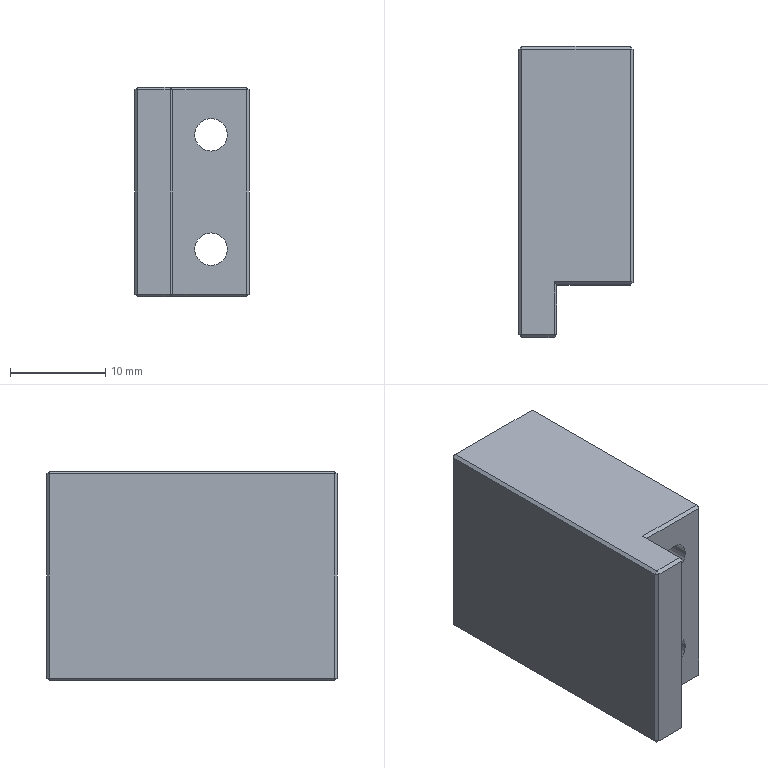Part | NX | features BREP 1 | 1 solid | 43 faces | box 12 x 30.5 x 22 mm | volume 6571 mm3 | plane 35 | cone 4 | cylinder 4 | commonest cylinder face diameters 3.4 x4
STEP:
#1=CARTESIAN_POINT('',(-3.7,-5.2,11.));
#2=VERTEX_POINT('',#1);
#3=CARTESIAN_POINT('',(-3.7,-5.5,10.7));
#4=VERTEX_POINT('',#3);
#5=CARTESIAN_POINT('',(-3.7,-5.5,10.7));
#6=DIRECTION('',(0.,-0.7071,-0.7071));
#7=VECTOR('',#6,1000.);
#8=LINE('',#5,#7);
#9=EDGE_CURVE('',#2,#4,#8,.T.);
#10=ORIENTED_EDGE('',*,*,#9,.T.);
#11=CARTESIAN_POINT('',(-0.3,-5.5,10.7));
#12=VERTEX_POINT('',#11);
#13=CARTESIAN_POINT('',(-4.,-5.5,10.7));
#14=DIRECTION('',(-1.,0.,0.));
#15=VECTOR('',#14,1000.);
#16=LINE('',#13,#15);
#17=EDGE_CURVE('',#12,#4,#16,.T.);
#18=ORIENTED_EDGE('',*,*,#17,.F.);
#19=CARTESIAN_POINT('',(-0.3,-5.2,11.));
#20=VERTEX_POINT('',#19);
#21=CARTESIAN_POINT('',(-0.3,-5.2,11.));
#22=DIRECTION('',(0.,0.7071,0.7071));
#23=VECTOR('',#22,1000.);
#24=LINE('',#21,#23);
#25=EDGE_CURVE('',#12,#20,#24,.T.);
#26=ORIENTED_EDGE('',*,*,#25,.T.);
#27=CARTESIAN_POINT('',(0.,-5.2,11.));
#28=DIRECTION('',(1.,0.,0.));
#29=VECTOR('',#28,1000.);
#30=LINE('',#27,#29);
#31=EDGE_CURVE('',#2,#20,#30,.T.);
#32=ORIENTED_EDGE('',*,*,#31,.F.);
#33=EDGE_LOOP('',(#10,#18,#26,#32));
#34=FACE_BOUND('',#33,.T.);
#35=CARTESIAN_POINT('',(0.,-5.2,11.));
#36=DIRECTION('',(0.,0.7071,-0.7071));
#37=DIRECTION('',(1.,0.,0.));
#38=AXIS2_PLACEMENT_3D('',#35,#36,#37);
#39=PLANE('',#38);
#40=ADVANCED_FACE('',(#34),#39,.F.);
#41=CARTESIAN_POINT('',(0.,-5.2,10.7));
#42=VERTEX_POINT('',#41);
#43=CARTESIAN_POINT('',(-0.15,-5.35,10.7));
#44=DIRECTION('',(0.7071,0.7071,0.));
#45=VECTOR('',#44,1000.);
#46=LINE('',#43,#45);
#47=EDGE_CURVE('',#12,#42,#46,.T.);
#48=ORIENTED_EDGE('',*,*,#47,.T.);
#49=CARTESIAN_POINT('',(-0.3,-5.2,11.));
#50=DIRECTION('',(-0.7071,0.,0.7071));
#51=VECTOR('',#50,1000.);
#52=LINE('',#49,#51);
#53=EDGE_CURVE('',#42,#20,#52,.T.);
#54=ORIENTED_EDGE('',*,*,#53,.T.);
#55=ORIENTED_EDGE('',*,*,#25,.F.);
#56=EDGE_LOOP('',(#48,#54,#55));
#57=FACE_BOUND('',#56,.T.);
#58=CARTESIAN_POINT('',(-0.3,-5.2,11.));
#59=DIRECTION('',(0.5774,-0.5774,0.5774));
#60=DIRECTION('',(0.7071,0.,-0.7071));
#61=AXIS2_PLACEMENT_3D('',#58,#59,#60);
#62=PLANE('',#61);
#63=ADVANCED_FACE('',(#57),#62,.T.);
#64=CARTESIAN_POINT('',(-4.,-5.2,10.7));
#65=VERTEX_POINT('',#64);
#66=CARTESIAN_POINT('',(-3.85,-5.2,10.85));
#67=DIRECTION('',(-0.7071,0.,-0.7071));
#68=VECTOR('',#67,1000.);
#69=LINE('',#66,#68);
#70=EDGE_CURVE('',#2,#65,#69,.T.);
#71=ORIENTED_EDGE('',*,*,#70,.T.);
#72=CARTESIAN_POINT('',(-3.7,-5.5,10.7));
#73=DIRECTION('',(0.7071,-0.7071,0.));
#74=VECTOR('',#73,1000.);
#75=LINE('',#72,#74);
#76=EDGE_CURVE('',#65,#4,#75,.T.);
#77=ORIENTED_EDGE('',*,*,#76,.T.);
#78=ORIENTED_EDGE('',*,*,#9,.F.);
#79=EDGE_LOOP('',(#71,#77,#78));
#80=FACE_BOUND('',#79,.T.);
#81=CARTESIAN_POINT('',(-3.7,-5.5,10.7));
#82=DIRECTION('',(-0.5774,-0.5774,0.5774));
#83=DIRECTION('',(0.7071,0.,0.7071));
#84=AXIS2_PLACEMENT_3D('',#81,#82,#83);
#85=PLANE('',#84);
#86=ADVANCED_FACE('',(#80),#85,.T.);
#87=CARTESIAN_POINT('',(-0.3,-5.5,-10.7));
#88=VERTEX_POINT('',#87);
#89=CARTESIAN_POINT('',(0.,-5.2,-10.7));
#90=VERTEX_POINT('',#89);
#91=CARTESIAN_POINT('',(-0.15,-5.35,-10.7));
#92=DIRECTION('',(0.7071,0.7071,0.));
#93=VECTOR('',#92,1000.);
#94=LINE('',#91,#93);
#95=EDGE_CURVE('',#88,#90,#94,.T.);
#96=ORIENTED_EDGE('',*,*,#95,.T.);
#97=CARTESIAN_POINT('',(0.,-5.2,11.));
#98=DIRECTION('',(0.,0.,-1.));
#99=VECTOR('',#98,1000.);
#100=LINE('',#97,#99);
#101=EDGE_CURVE('',#42,#90,#100,.T.);
#102=ORIENTED_EDGE('',*,*,#101,.F.);
#103=ORIENTED_EDGE('',*,*,#47,.F.);
#104=CARTESIAN_POINT('',(-0.3,-5.5,11.));
#105=DIRECTION('',(0.,0.,1.));
#106=VECTOR('',#105,1000.);
#107=LINE('',#104,#106);
#108=EDGE_CURVE('',#88,#12,#107,.T.);
#109=ORIENTED_EDGE('',*,*,#108,.F.);
#110=EDGE_LOOP('',(#96,#102,#103,#109));
#111=FACE_BOUND('',#110,.T.);
#112=CARTESIAN_POINT('',(0.,-5.2,11.));
#113=DIRECTION('',(-0.7071,0.7071,0.));
#114=DIRECTION('',(0.,0.,-1.));
#115=AXIS2_PLACEMENT_3D('',#112,#113,#114);
#116=PLANE('',#115);
#117=ADVANCED_FACE('',(#111),#116,.F.);
#118=CARTESIAN_POINT('',(0.,0.,10.7));
#119=VERTEX_POINT('',#118);
#120=CARTESIAN_POINT('',(-0.3,0.3,11.));
#121=VERTEX_POINT('',#120);
#122=CARTESIAN_POINT('',(-0.2,0.2,10.9));
#123=DIRECTION('',(-0.5774,0.5774,0.5774));
#124=VECTOR('',#123,1000.);
#125=LINE('',#122,#124);
#126=EDGE_CURVE('',#119,#121,#125,.T.);
#127=ORIENTED_EDGE('',*,*,#126,.T.);
#128=CARTESIAN_POINT('',(-0.3,0.,11.));
#129=DIRECTION('',(0.,1.,0.));
#130=VECTOR('',#129,1000.);
#131=LINE('',#128,#130);
#132=EDGE_CURVE('',#20,#121,#131,.T.);
#133=ORIENTED_EDGE('',*,*,#132,.F.);
#134=ORIENTED_EDGE('',*,*,#53,.F.);
#135=CARTESIAN_POINT('',(0.,-5.5,10.7));
#136=DIRECTION('',(0.,-1.,0.));
#137=VECTOR('',#136,1000.);
#138=LINE('',#135,#137);
#139=EDGE_CURVE('',#119,#42,#138,.T.);
#140=ORIENTED_EDGE('',*,*,#139,.F.);
#141=EDGE_LOOP('',(#127,#133,#134,#140));
#142=FACE_BOUND('',#141,.T.);
#143=CARTESIAN_POINT('',(-0.3,0.,11.));
#144=DIRECTION('',(-0.7071,0.,-0.7071));
#145=DIRECTION('',(0.,1.,0.));
#146=AXIS2_PLACEMENT_3D('',#143,#144,#145);
#147=PLANE('',#146);
#148=ADVANCED_FACE('',(#142),#147,.F.);
#149=CARTESIAN_POINT('',(-3.7,24.7,11.));
#150=VERTEX_POINT('',#149);
#151=CARTESIAN_POINT('',(-4.,24.7,10.7));
#152=VERTEX_POINT('',#151);
#153=CARTESIAN_POINT('',(-3.7,24.7,11.));
#154=DIRECTION('',(-0.7071,0.,-0.7071));
#155=VECTOR('',#154,1000.);
#156=LINE('',#153,#155);
#157=EDGE_CURVE('',#150,#152,#156,.T.);
#158=ORIENTED_EDGE('',*,*,#157,.T.);
#159=CARTESIAN_POINT('',(-4.,25.,10.7));
#160=DIRECTION('',(0.,1.,0.));
#161=VECTOR('',#160,1000.);
#162=LINE('',#159,#161);
#163=EDGE_CURVE('',#65,#152,#162,.T.);
#164=ORIENTED_EDGE('',*,*,#163,.F.);
#165=ORIENTED_EDGE('',*,*,#70,.F.);
#166=CARTESIAN_POINT('',(-3.7,0.,11.));
#167=DIRECTION('',(0.,-1.,0.));
#168=VECTOR('',#167,1000.);
#169=LINE('',#166,#168);
#170=EDGE_CURVE('',#150,#2,#169,.T.);
#171=ORIENTED_EDGE('',*,*,#170,.F.);
#172=EDGE_LOOP('',(#158,#164,#165,#171));
#173=FACE_BOUND('',#172,.T.);
#174=CARTESIAN_POINT('',(-3.7,0.,11.));
#175=DIRECTION('',(0.7071,0.,-0.7071));
#176=DIRECTION('',(0.,-1.,0.));
#177=AXIS2_PLACEMENT_3D('',#174,#175,#176);
#178=PLANE('',#177);
#179=ADVANCED_FACE('',(#173),#178,.F.);
#180=CARTESIAN_POINT('',(-4.,-5.2,-10.7));
#181=VERTEX_POINT('',#180);
#182=CARTESIAN_POINT('',(-3.7,-5.5,-10.7));
#183=VERTEX_POINT('',#182);
#184=CARTESIAN_POINT('',(-3.85,-5.35,-10.7));
#185=DIRECTION('',(0.7071,-0.7071,0.));
#186=VECTOR('',#185,1000.);
#187=LINE('',#184,#186);
#188=EDGE_CURVE('',#181,#183,#187,.T.);
#189=ORIENTED_EDGE('',*,*,#188,.T.);
#190=CARTESIAN_POINT('',(-3.7,-5.5,11.));
#191=DIRECTION('',(0.,0.,-1.));
#192=VECTOR('',#191,1000.);
#193=LINE('',#190,#192);
#194=EDGE_CURVE('',#4,#183,#193,.T.);
#195=ORIENTED_EDGE('',*,*,#194,.F.);
#196=ORIENTED_EDGE('',*,*,#76,.F.);
#197=CARTESIAN_POINT('',(-4.,-5.2,11.));
#198=DIRECTION('',(0.,0.,1.));
#199=VECTOR('',#198,1000.);
#200=LINE('',#197,#199);
#201=EDGE_CURVE('',#181,#65,#200,.T.);
#202=ORIENTED_EDGE('',*,*,#201,.F.);
#203=EDGE_LOOP('',(#189,#195,#196,#202));
#204=FACE_BOUND('',#203,.T.);
#205=CARTESIAN_POINT('',(-3.7,-5.5,11.));
#206=DIRECTION('',(0.7071,0.7071,0.));
#207=DIRECTION('',(0.,0.,-1.));
#208=AXIS2_PLACEMENT_3D('',#205,#206,#207);
#209=PLANE('',#208);
#210=ADVANCED_FACE('',(#204),#209,.F.);
#211=CARTESIAN_POINT('',(-0.3,-5.2,-11.));
#212=VERTEX_POINT('',#211);
#213=CARTESIAN_POINT('',(-0.3,-5.2,-11.));
#214=DIRECTION('',(0.,0.7071,-0.7071));
#215=VECTOR('',#214,1000.);
#216=LINE('',#213,#215);
#217=EDGE_CURVE('',#88,#212,#216,.T.);
#218=ORIENTED_EDGE('',*,*,#217,.T.);
#219=CARTESIAN_POINT('',(-0.3,-5.2,-11.));
#220=DIRECTION('',(0.7071,0.,0.7071));
#221=VECTOR('',#220,1000.);
#222=LINE('',#219,#221);
#223=EDGE_CURVE('',#212,#90,#222,.T.);
#224=ORIENTED_EDGE('',*,*,#223,.T.);
#225=ORIENTED_EDGE('',*,*,#95,.F.);
#226=EDGE_LOOP('',(#218,#224,#225));
#227=FACE_BOUND('',#226,.T.);
#228=CARTESIAN_POINT('',(-0.3,-5.2,-11.));
#229=DIRECTION('',(0.5774,-0.5774,-0.5774));
#230=DIRECTION('',(-0.7071,0.,-0.7071));
#231=AXIS2_PLACEMENT_3D('',#228,#229,#230);
#232=PLANE('',#231);
#233=ADVANCED_FACE('',(#227),#232,.T.);
#234=CARTESIAN_POINT('',(7.7,0.,10.7));
#235=VERTEX_POINT('',#234);
#236=CARTESIAN_POINT('',(7.7,0.3,11.));
#237=VERTEX_POINT('',#236);
#238=CARTESIAN_POINT('',(7.7,0.15,10.85));
#239=DIRECTION('',(0.,0.7071,0.7071));
#240=VECTOR('',#239,1000.);
#241=LINE('',#238,#240);
#242=EDGE_CURVE('',#235,#237,#241,.T.);
#243=ORIENTED_EDGE('',*,*,#242,.T.);
#244=CARTESIAN_POINT('',(0.,0.3,11.));
#245=DIRECTION('',(1.,0.,0.));
#246=VECTOR('',#245,1000.);
#247=LINE('',#244,#246);
#248=EDGE_CURVE('',#121,#237,#247,.T.);
#249=ORIENTED_EDGE('',*,*,#248,.F.);
#250=ORIENTED_EDGE('',*,*,#126,.F.);
#251=CARTESIAN_POINT('',(0.,0.,10.7));
#252=DIRECTION('',(-1.,0.,0.));
#253=VECTOR('',#252,1000.);
#254=LINE('',#251,#253);
#255=EDGE_CURVE('',#235,#119,#254,.T.);
#256=ORIENTED_EDGE('',*,*,#255,.F.);
#257=EDGE_LOOP('',(#243,#249,#250,#256));
#258=FACE_BOUND('',#257,.T.);
#259=CARTESIAN_POINT('',(0.,0.3,11.));
#260=DIRECTION('',(0.,0.7071,-0.7071));
#261=DIRECTION('',(1.,0.,0.));
#262=AXIS2_PLACEMENT_3D('',#259,#260,#261);
#263=PLANE('',#262);
#264=ADVANCED_FACE('',(#258),#263,.F.);
#265=CARTESIAN_POINT('',(-3.7,25.,10.7));
#266=VERTEX_POINT('',#265);
#267=CARTESIAN_POINT('',(-3.7,24.7,11.));
#268=DIRECTION('',(0.,0.7071,-0.7071));
#269=VECTOR('',#268,1000.);
#270=LINE('',#267,#269);
#271=EDGE_CURVE('',#150,#266,#270,.T.);
#272=ORIENTED_EDGE('',*,*,#271,.T.);
#273=CARTESIAN_POINT('',(-3.85,24.85,10.7));
#274=DIRECTION('',(-0.7071,-0.7071,0.));
#275=VECTOR('',#274,1000.);
#276=LINE('',#273,#275);
#277=EDGE_CURVE('',#266,#152,#276,.T.);
#278=ORIENTED_EDGE('',*,*,#277,.T.);
#279=ORIENTED_EDGE('',*,*,#157,.F.);
#280=EDGE_LOOP('',(#272,#278,#279));
#281=FACE_BOUND('',#280,.T.);
#282=CARTESIAN_POINT('',(-3.7,24.7,11.));
#283=DIRECTION('',(-0.5774,0.5774,0.5774));
#284=DIRECTION('',(0.7071,0.,0.7071));
#285=AXIS2_PLACEMENT_3D('',#282,#283,#284);
#286=PLANE('',#285);
#287=ADVANCED_FACE('',(#281),#286,.T.);
#288=CARTESIAN_POINT('',(-3.7,-5.2,-11.));
#289=VERTEX_POINT('',#288);
#290=CARTESIAN_POINT('',(-3.7,-5.2,-11.));
#291=DIRECTION('',(0.7071,0.,-0.7071));
#292=VECTOR('',#291,1000.);
#293=LINE('',#290,#292);
#294=EDGE_CURVE('',#181,#289,#293,.T.);
#295=ORIENTED_EDGE('',*,*,#294,.T.);
#296=CARTESIAN_POINT('',(-3.7,-5.2,-11.));
#297=DIRECTION('',(0.,-0.7071,0.7071));
#298=VECTOR('',#297,1000.);
#299=LINE('',#296,#298);
#300=EDGE_CURVE('',#289,#183,#299,.T.);
#301=ORIENTED_EDGE('',*,*,#300,.T.);
#302=ORIENTED_EDGE('',*,*,#188,.F.);
#303=EDGE_LOOP('',(#295,#301,#302));
#304=FACE_BOUND('',#303,.T.);
#305=CARTESIAN_POINT('',(-3.7,-5.2,-11.));
#306=DIRECTION('',(-0.5774,-0.5774,-0.5774));
#307=DIRECTION('',(-0.7071,0.,0.7071));
#308=AXIS2_PLACEMENT_3D('',#305,#306,#307);
#309=PLANE('',#308);
#310=ADVANCED_FACE('',(#304),#309,.T.);
#311=ORIENTED_EDGE('',*,*,#300,.F.);
#312=CARTESIAN_POINT('',(-4.,-5.2,-11.));
#313=DIRECTION('',(-1.,0.,0.));
#314=VECTOR('',#313,1000.);
#315=LINE('',#312,#314);
#316=EDGE_CURVE('',#212,#289,#315,.T.);
#317=ORIENTED_EDGE('',*,*,#316,.F.);
#318=ORIENTED_EDGE('',*,*,#217,.F.);
#319=CARTESIAN_POINT('',(0.,-5.5,-10.7));
#320=DIRECTION('',(1.,0.,0.));
#321=VECTOR('',#320,1000.);
#322=LINE('',#319,#321);
#323=EDGE_CURVE('',#183,#88,#322,.T.);
#324=ORIENTED_EDGE('',*,*,#323,.F.);
#325=EDGE_LOOP('',(#311,#317,#318,#324));
#326=FACE_BOUND('',#325,.T.);
#327=CARTESIAN_POINT('',(-4.,-5.5,-10.7));
#328=DIRECTION('',(0.,-0.7071,-0.7071));
#329=DIRECTION('',(-1.,0.,0.));
#330=AXIS2_PLACEMENT_3D('',#327,#328,#329);
#331=PLANE('',#330);
#332=ADVANCED_FACE('',(#326),#331,.T.);
#333=CARTESIAN_POINT('',(-0.3,0.3,-11.));
#334=VERTEX_POINT('',#333);
#335=CARTESIAN_POINT('',(0.,0.,-10.7));
#336=VERTEX_POINT('',#335);
#337=CARTESIAN_POINT('',(0.,0.,-10.7));
#338=DIRECTION('',(0.5774,-0.5774,0.5774));
#339=VECTOR('',#338,1000.);
#340=LINE('',#337,#339);
#341=EDGE_CURVE('',#334,#336,#340,.T.);
#342=ORIENTED_EDGE('',*,*,#341,.T.);
#343=CARTESIAN_POINT('',(0.,0.,-10.7));
#344=DIRECTION('',(0.,1.,0.));
#345=VECTOR('',#344,1000.);
#346=LINE('',#343,#345);
#347=EDGE_CURVE('',#90,#336,#346,.T.);
#348=ORIENTED_EDGE('',*,*,#347,.F.);
#349=ORIENTED_EDGE('',*,*,#223,.F.);
#350=CARTESIAN_POINT('',(-0.3,-5.5,-11.));
#351=DIRECTION('',(0.,-1.,0.));
#352=VECTOR('',#351,1000.);
#353=LINE('',#350,#352);
#354=EDGE_CURVE('',#334,#212,#353,.T.);
#355=ORIENTED_EDGE('',*,*,#354,.F.);
#356=EDGE_LOOP('',(#342,#348,#349,#355));
#357=FACE_BOUND('',#356,.T.);
#358=CARTESIAN_POINT('',(0.,-5.5,-10.7));
#359=DIRECTION('',(0.7071,0.,-0.7071));
#360=DIRECTION('',(0.,-1.,0.));
#361=AXIS2_PLACEMENT_3D('',#358,#359,#360);
#362=PLANE('',#361);
#363=ADVANCED_FACE('',(#357),#362,.T.);
#364=CARTESIAN_POINT('',(8.,0.3,10.7));
#365=VERTEX_POINT('',#364);
#366=CARTESIAN_POINT('',(8.,0.3,10.7));
#367=DIRECTION('',(0.7071,0.7071,0.));
#368=VECTOR('',#367,1000.);
#369=LINE('',#366,#368);
#370=EDGE_CURVE('',#235,#365,#369,.T.);
#371=ORIENTED_EDGE('',*,*,#370,.T.);
#372=CARTESIAN_POINT('',(8.,0.3,10.7));
#373=DIRECTION('',(-0.7071,0.,0.7071));
#374=VECTOR('',#373,1000.);
#375=LINE('',#372,#374);
#376=EDGE_CURVE('',#365,#237,#375,.T.);
#377=ORIENTED_EDGE('',*,*,#376,.T.);
#378=ORIENTED_EDGE('',*,*,#242,.F.);
#379=EDGE_LOOP('',(#371,#377,#378));
#380=FACE_BOUND('',#379,.T.);
#381=CARTESIAN_POINT('',(8.,0.3,10.7));
#382=DIRECTION('',(0.5774,-0.5774,0.5774));
#383=DIRECTION('',(0.7071,0.,-0.7071));
#384=AXIS2_PLACEMENT_3D('',#381,#382,#383);
#385=PLANE('',#384);
#386=ADVANCED_FACE('',(#380),#385,.T.);
#387=CARTESIAN_POINT('',(7.7,24.7,11.));
#388=VERTEX_POINT('',#387);
#389=CARTESIAN_POINT('',(7.7,25.,10.7));
#390=VERTEX_POINT('',#389);
#391=CARTESIAN_POINT('',(7.7,25.,10.7));
#392=DIRECTION('',(0.,0.7071,-0.7071));
#393=VECTOR('',#392,1000.);
#394=LINE('',#391,#393);
#395=EDGE_CURVE('',#388,#390,#394,.T.);
#396=ORIENTED_EDGE('',*,*,#395,.T.);
#397=CARTESIAN_POINT('',(8.,25.,10.7));
#398=DIRECTION('',(1.,0.,0.));
#399=VECTOR('',#398,1000.);
#400=LINE('',#397,#399);
#401=EDGE_CURVE('',#266,#390,#400,.T.);
#402=ORIENTED_EDGE('',*,*,#401,.F.);
#403=ORIENTED_EDGE('',*,*,#271,.F.);
#404=CARTESIAN_POINT('',(0.,24.7,11.));
#405=DIRECTION('',(-1.,0.,0.));
#406=VECTOR('',#405,1000.);
#407=LINE('',#404,#406);
#408=EDGE_CURVE('',#388,#150,#407,.T.);
#409=ORIENTED_EDGE('',*,*,#408,.F.);
#410=EDGE_LOOP('',(#396,#402,#403,#409));
#411=FACE_BOUND('',#410,.T.);
#412=CARTESIAN_POINT('',(0.,24.7,11.));
#413=DIRECTION('',(0.,-0.7071,-0.7071));
#414=DIRECTION('',(-1.,0.,0.));
#415=AXIS2_PLACEMENT_3D('',#412,#413,#414);
#416=PLANE('',#415);
#417=ADVANCED_FACE('',(#411),#416,.F.);
#418=CARTESIAN_POINT('',(-3.7,25.,-10.7));
#419=VERTEX_POINT('',#418);
#420=CARTESIAN_POINT('',(-4.,24.7,-10.7));
#421=VERTEX_POINT('',#420);
#422=CARTESIAN_POINT('',(-4.,24.7,-10.7));
#423=DIRECTION('',(-0.7071,-0.7071,0.));
#424=VECTOR('',#423,1000.);
#425=LINE('',#422,#424);
#426=EDGE_CURVE('',#419,#421,#425,.T.);
#427=ORIENTED_EDGE('',*,*,#426,.T.);
#428=CARTESIAN_POINT('',(-4.,24.7,11.));
#429=DIRECTION('',(0.,0.,-1.));
#430=VECTOR('',#429,1000.);
#431=LINE('',#428,#430);
#432=EDGE_CURVE('',#152,#421,#431,.T.);
#433=ORIENTED_EDGE('',*,*,#432,.F.);
#434=ORIENTED_EDGE('',*,*,#277,.F.);
#435=CARTESIAN_POINT('',(-3.7,25.,11.));
#436=DIRECTION('',(0.,0.,1.));
#437=VECTOR('',#436,1000.);
#438=LINE('',#435,#437);
#439=EDGE_CURVE('',#419,#266,#438,.T.);
#440=ORIENTED_EDGE('',*,*,#439,.F.);
#441=EDGE_LOOP('',(#427,#433,#434,#440));
#442=FACE_BOUND('',#441,.T.);
#443=CARTESIAN_POINT('',(-4.,24.7,11.));
#444=DIRECTION('',(0.7071,-0.7071,0.));
#445=DIRECTION('',(0.,0.,-1.));
#446=AXIS2_PLACEMENT_3D('',#443,#444,#445);
#447=PLANE('',#446);
#448=ADVANCED_FACE('',(#442),#447,.F.);
#449=CARTESIAN_POINT('',(-3.7,24.7,-11.));
#450=VERTEX_POINT('',#449);
#451=CARTESIAN_POINT('',(-4.,24.7,-10.7));
#452=DIRECTION('',(0.7071,0.,-0.7071));
#453=VECTOR('',#452,1000.);
#454=LINE('',#451,#453);
#455=EDGE_CURVE('',#421,#450,#454,.T.);
#456=ORIENTED_EDGE('',*,*,#455,.T.);
#457=CARTESIAN_POINT('',(-3.7,25.,-11.));
#458=DIRECTION('',(0.,1.,0.));
#459=VECTOR('',#458,1000.);
#460=LINE('',#457,#459);
#461=EDGE_CURVE('',#289,#450,#460,.T.);
#462=ORIENTED_EDGE('',*,*,#461,.F.);
#463=ORIENTED_EDGE('',*,*,#294,.F.);
#464=CARTESIAN_POINT('',(-4.,-5.5,-10.7));
#465=DIRECTION('',(0.,-1.,0.));
#466=VECTOR('',#465,1000.);
#467=LINE('',#464,#466);
#468=EDGE_CURVE('',#421,#181,#467,.T.);
#469=ORIENTED_EDGE('',*,*,#468,.F.);
#470=EDGE_LOOP('',(#456,#462,#463,#469));
#471=FACE_BOUND('',#470,.T.);
#472=CARTESIAN_POINT('',(-4.,25.,-10.7));
#473=DIRECTION('',(-0.7071,0.,-0.7071));
#474=DIRECTION('',(0.,1.,0.));
#475=AXIS2_PLACEMENT_3D('',#472,#473,#474);
#476=PLANE('',#475);
#477=ADVANCED_FACE('',(#471),#476,.T.);
#478=CARTESIAN_POINT('',(7.7,0.3,-11.));
#479=VERTEX_POINT('',#478);
#480=CARTESIAN_POINT('',(7.7,0.,-10.7));
#481=VERTEX_POINT('',#480);
#482=CARTESIAN_POINT('',(7.7,0.,-10.7));
#483=DIRECTION('',(0.,-0.7071,0.7071));
#484=VECTOR('',#483,1000.);
#485=LINE('',#482,#484);
#486=EDGE_CURVE('',#479,#481,#485,.T.);
#487=ORIENTED_EDGE('',*,*,#486,.T.);
#488=CARTESIAN_POINT('',(8.,0.,-10.7));
#489=DIRECTION('',(1.,0.,0.));
#490=VECTOR('',#489,1000.);
#491=LINE('',#488,#490);
#492=EDGE_CURVE('',#336,#481,#491,.T.);
#493=ORIENTED_EDGE('',*,*,#492,.F.);
#494=ORIENTED_EDGE('',*,*,#341,.F.);
#495=CARTESIAN_POINT('',(0.,0.3,-11.));
#496=DIRECTION('',(-1.,0.,0.));
#497=VECTOR('',#496,1000.);
#498=LINE('',#495,#497);
#499=EDGE_CURVE('',#479,#334,#498,.T.);
#500=ORIENTED_EDGE('',*,*,#499,.F.);
#501=EDGE_LOOP('',(#487,#493,#494,#500));
#502=FACE_BOUND('',#501,.T.);
#503=CARTESIAN_POINT('',(0.,0.,-10.7));
#504=DIRECTION('',(0.,-0.7071,-0.7071));
#505=DIRECTION('',(-1.,0.,0.));
#506=AXIS2_PLACEMENT_3D('',#503,#504,#505);
#507=PLANE('',#506);
#508=ADVANCED_FACE('',(#502),#507,.T.);
#509=CARTESIAN_POINT('',(8.,0.3,-10.7));
#510=VERTEX_POINT('',#509);
#511=CARTESIAN_POINT('',(7.7,0.,-10.7));
#512=DIRECTION('',(0.7071,0.7071,0.));
#513=VECTOR('',#512,1000.);
#514=LINE('',#511,#513);
#515=EDGE_CURVE('',#481,#510,#514,.T.);
#516=ORIENTED_EDGE('',*,*,#515,.T.);
#517=CARTESIAN_POINT('',(8.,0.3,11.));
#518=DIRECTION('',(0.,0.,-1.));
#519=VECTOR('',#518,1000.);
#520=LINE('',#517,#519);
#521=EDGE_CURVE('',#365,#510,#520,.T.);
#522=ORIENTED_EDGE('',*,*,#521,.F.);
#523=ORIENTED_EDGE('',*,*,#370,.F.);
#524=CARTESIAN_POINT('',(7.7,0.,11.));
#525=DIRECTION('',(0.,0.,1.));
#526=VECTOR('',#525,1000.);
#527=LINE('',#524,#526);
#528=EDGE_CURVE('',#481,#235,#527,.T.);
#529=ORIENTED_EDGE('',*,*,#528,.F.);
#530=EDGE_LOOP('',(#516,#522,#523,#529));
#531=FACE_BOUND('',#530,.T.);
#532=CARTESIAN_POINT('',(8.,0.3,11.));
#533=DIRECTION('',(-0.7071,0.7071,0.));
#534=DIRECTION('',(0.,0.,-1.));
#535=AXIS2_PLACEMENT_3D('',#532,#533,#534);
#536=PLANE('',#535);
#537=ADVANCED_FACE('',(#531),#536,.F.);
#538=CARTESIAN_POINT('',(8.,24.7,10.7));
#539=VERTEX_POINT('',#538);
#540=CARTESIAN_POINT('',(7.85,24.7,10.85));
#541=DIRECTION('',(-0.7071,0.,0.7071));
#542=VECTOR('',#541,1000.);
#543=LINE('',#540,#542);
#544=EDGE_CURVE('',#539,#388,#543,.T.);
#545=ORIENTED_EDGE('',*,*,#544,.T.);
#546=CARTESIAN_POINT('',(7.7,0.,11.));
#547=DIRECTION('',(0.,1.,0.));
#548=VECTOR('',#547,1000.);
#549=LINE('',#546,#548);
#550=EDGE_CURVE('',#237,#388,#549,.T.);
#551=ORIENTED_EDGE('',*,*,#550,.F.);
#552=ORIENTED_EDGE('',*,*,#376,.F.);
#553=CARTESIAN_POINT('',(8.,0.,10.7));
#554=DIRECTION('',(0.,-1.,0.));
#555=VECTOR('',#554,1000.);
#556=LINE('',#553,#555);
#557=EDGE_CURVE('',#539,#365,#556,.T.);
#558=ORIENTED_EDGE('',*,*,#557,.F.);
#559=EDGE_LOOP('',(#545,#551,#552,#558));
#560=FACE_BOUND('',#559,.T.);
#561=CARTESIAN_POINT('',(7.7,0.,11.));
#562=DIRECTION('',(-0.7071,0.,-0.7071));
#563=DIRECTION('',(0.,1.,0.));
#564=AXIS2_PLACEMENT_3D('',#561,#562,#563);
#565=PLANE('',#564);
#566=ADVANCED_FACE('',(#560),#565,.F.);
#567=ORIENTED_EDGE('',*,*,#395,.F.);
#568=ORIENTED_EDGE('',*,*,#544,.F.);
#569=CARTESIAN_POINT('',(7.7,25.,10.7));
#570=DIRECTION('',(-0.7071,0.7071,0.));
#571=VECTOR('',#570,1000.);
#572=LINE('',#569,#571);
#573=EDGE_CURVE('',#539,#390,#572,.T.);
#574=ORIENTED_EDGE('',*,*,#573,.T.);
#575=EDGE_LOOP('',(#567,#568,#574));
#576=FACE_BOUND('',#575,.T.);
#577=CARTESIAN_POINT('',(7.7,25.,10.7));
#578=DIRECTION('',(0.5774,0.5774,0.5774));
#579=DIRECTION('',(0.7071,0.,-0.7071));
#580=AXIS2_PLACEMENT_3D('',#577,#578,#579);
#581=PLANE('',#580);
#582=ADVANCED_FACE('',(#576),#581,.T.);
#583=ORIENTED_EDGE('',*,*,#426,.F.);
#584=CARTESIAN_POINT('',(-3.7,24.85,-10.85));
#585=DIRECTION('',(0.,-0.7071,-0.7071));
#586=VECTOR('',#585,1000.);
#587=LINE('',#584,#586);
#588=EDGE_CURVE('',#419,#450,#587,.T.);
#589=ORIENTED_EDGE('',*,*,#588,.T.);
#590=ORIENTED_EDGE('',*,*,#455,.F.);
#591=EDGE_LOOP('',(#583,#589,#590));
#592=FACE_BOUND('',#591,.T.);
#593=CARTESIAN_POINT('',(-4.,24.7,-10.7));
#594=DIRECTION('',(-0.5774,0.5774,-0.5774));
#595=DIRECTION('',(-0.7071,0.,0.7071));
#596=AXIS2_PLACEMENT_3D('',#593,#594,#595);
#597=PLANE('',#596);
#598=ADVANCED_FACE('',(#592),#597,.T.);
#599=ORIENTED_EDGE('',*,*,#486,.F.);
#600=CARTESIAN_POINT('',(7.85,0.3,-10.85));
#601=DIRECTION('',(0.7071,0.,0.7071));
#602=VECTOR('',#601,1000.);
#603=LINE('',#600,#602);
#604=EDGE_CURVE('',#479,#510,#603,.T.);
#605=ORIENTED_EDGE('',*,*,#604,.T.);
#606=ORIENTED_EDGE('',*,*,#515,.F.);
#607=EDGE_LOOP('',(#599,#605,#606));
#608=FACE_BOUND('',#607,.T.);
#609=CARTESIAN_POINT('',(7.7,0.,-10.7));
#610=DIRECTION('',(0.5774,-0.5774,-0.5774));
#611=DIRECTION('',(-0.7071,0.,-0.7071));
#612=AXIS2_PLACEMENT_3D('',#609,#610,#611);
#613=PLANE('',#612);
#614=ADVANCED_FACE('',(#608),#613,.T.);
#615=CARTESIAN_POINT('',(8.,24.7,-10.7));
#616=VERTEX_POINT('',#615);
#617=CARTESIAN_POINT('',(7.7,25.,-10.7));
#618=VERTEX_POINT('',#617);
#619=CARTESIAN_POINT('',(7.85,24.85,-10.7));
#620=DIRECTION('',(-0.7071,0.7071,0.));
#621=VECTOR('',#620,1000.);
#622=LINE('',#619,#621);
#623=EDGE_CURVE('',#616,#618,#622,.T.);
#624=ORIENTED_EDGE('',*,*,#623,.T.);
#625=CARTESIAN_POINT('',(7.7,25.,11.));
#626=DIRECTION('',(0.,0.,-1.));
#627=VECTOR('',#626,1000.);
#628=LINE('',#625,#627);
#629=EDGE_CURVE('',#390,#618,#628,.T.);
#630=ORIENTED_EDGE('',*,*,#629,.F.);
#631=ORIENTED_EDGE('',*,*,#573,.F.);
#632=CARTESIAN_POINT('',(8.,24.7,11.));
#633=DIRECTION('',(0.,0.,1.));
#634=VECTOR('',#633,1000.);
#635=LINE('',#632,#634);
#636=EDGE_CURVE('',#616,#539,#635,.T.);
#637=ORIENTED_EDGE('',*,*,#636,.F.);
#638=EDGE_LOOP('',(#624,#630,#631,#637));
#639=FACE_BOUND('',#638,.T.);
#640=CARTESIAN_POINT('',(7.7,25.,11.));
#641=DIRECTION('',(-0.7071,-0.7071,0.));
#642=DIRECTION('',(0.,0.,-1.));
#643=AXIS2_PLACEMENT_3D('',#640,#641,#642);
#644=PLANE('',#643);
#645=ADVANCED_FACE('',(#639),#644,.F.);
#646=CARTESIAN_POINT('',(7.7,24.7,-11.));
#647=VERTEX_POINT('',#646);
#648=CARTESIAN_POINT('',(7.7,24.7,-11.));
#649=DIRECTION('',(0.,-0.7071,-0.7071));
#650=VECTOR('',#649,1000.);
#651=LINE('',#648,#650);
#652=EDGE_CURVE('',#618,#647,#651,.T.);
#653=ORIENTED_EDGE('',*,*,#652,.T.);
#654=CARTESIAN_POINT('',(8.,24.7,-11.));
#655=DIRECTION('',(1.,0.,0.));
#656=VECTOR('',#655,1000.);
#657=LINE('',#654,#656);
#658=EDGE_CURVE('',#450,#647,#657,.T.);
#659=ORIENTED_EDGE('',*,*,#658,.F.);
#660=ORIENTED_EDGE('',*,*,#588,.F.);
#661=CARTESIAN_POINT('',(-4.,25.,-10.7));
#662=DIRECTION('',(-1.,0.,0.));
#663=VECTOR('',#662,1000.);
#664=LINE('',#661,#663);
#665=EDGE_CURVE('',#618,#419,#664,.T.);
#666=ORIENTED_EDGE('',*,*,#665,.F.);
#667=EDGE_LOOP('',(#653,#659,#660,#666));
#668=FACE_BOUND('',#667,.T.);
#669=CARTESIAN_POINT('',(8.,25.,-10.7));
#670=DIRECTION('',(0.,0.7071,-0.7071));
#671=DIRECTION('',(1.,0.,0.));
#672=AXIS2_PLACEMENT_3D('',#669,#670,#671);
#673=PLANE('',#672);
#674=ADVANCED_FACE('',(#668),#673,.T.);
#675=CARTESIAN_POINT('',(7.7,24.7,-11.));
#676=DIRECTION('',(0.7071,0.,0.7071));
#677=VECTOR('',#676,1000.);
#678=LINE('',#675,#677);
#679=EDGE_CURVE('',#647,#616,#678,.T.);
#680=ORIENTED_EDGE('',*,*,#679,.T.);
#681=CARTESIAN_POINT('',(8.,25.,-10.7));
#682=DIRECTION('',(0.,1.,0.));
#683=VECTOR('',#682,1000.);
#684=LINE('',#681,#683);
#685=EDGE_CURVE('',#510,#616,#684,.T.);
#686=ORIENTED_EDGE('',*,*,#685,.F.);
#687=ORIENTED_EDGE('',*,*,#604,.F.);
#688=CARTESIAN_POINT('',(7.7,0.,-11.));
#689=DIRECTION('',(0.,-1.,0.));
#690=VECTOR('',#689,1000.);
#691=LINE('',#688,#690);
#692=EDGE_CURVE('',#647,#479,#691,.T.);
#693=ORIENTED_EDGE('',*,*,#692,.F.);
#694=EDGE_LOOP('',(#680,#686,#687,#693));
#695=FACE_BOUND('',#694,.T.);
#696=CARTESIAN_POINT('',(8.,0.,-10.7));
#697=DIRECTION('',(0.7071,0.,-0.7071));
#698=DIRECTION('',(0.,-1.,0.));
#699=AXIS2_PLACEMENT_3D('',#696,#697,#698);
#700=PLANE('',#699);
#701=ADVANCED_FACE('',(#695),#700,.T.);
#702=ORIENTED_EDGE('',*,*,#623,.F.);
#703=ORIENTED_EDGE('',*,*,#679,.F.);
#704=ORIENTED_EDGE('',*,*,#652,.F.);
#705=EDGE_LOOP('',(#702,#703,#704));
#706=FACE_BOUND('',#705,.T.);
#707=CARTESIAN_POINT('',(7.7,24.7,-11.));
#708=DIRECTION('',(0.5774,0.5774,-0.5774));
#709=DIRECTION('',(-0.7071,0.,-0.7071));
#710=AXIS2_PLACEMENT_3D('',#707,#708,#709);
#711=PLANE('',#710);
#712=ADVANCED_FACE('',(#706),#711,.T.);
#713=CARTESIAN_POINT('',(4.,25.,2.5));
#714=VERTEX_POINT('',#713);
#715=CARTESIAN_POINT('',(4.,23.2,4.3));
#716=VERTEX_POINT('',#715);
#717=CARTESIAN_POINT('',(4.,25.,2.5));
#718=DIRECTION('',(0.,0.7071,-0.7071));
#719=VECTOR('',#718,1000.);
#720=LINE('',#717,#719);
#721=EDGE_CURVE('',#714,#716,#720,.F.);
#722=ORIENTED_EDGE('',*,*,#721,.T.);
#723=CARTESIAN_POINT('',(4.,23.2,7.7));
#724=VERTEX_POINT('',#723);
#725=CARTESIAN_POINT('',(4.,23.2,6.));
#726=DIRECTION('',(0.,1.,0.));
#727=DIRECTION('',(0.,0.,1.));
#728=AXIS2_PLACEMENT_3D('',#725,#726,#727);
#729=CIRCLE('',#728,1.7);
#730=EDGE_CURVE('',#724,#716,#729,.T.);
#731=ORIENTED_EDGE('',*,*,#730,.F.);
#732=CARTESIAN_POINT('',(4.,25.,9.5));
#733=VERTEX_POINT('',#732);
#734=CARTESIAN_POINT('',(4.,25.,9.5));
#735=DIRECTION('',(0.,0.7071,0.7071));
#736=VECTOR('',#735,1000.);
#737=LINE('',#734,#736);
#738=EDGE_CURVE('',#733,#724,#737,.F.);
#739=ORIENTED_EDGE('',*,*,#738,.F.);
#740=CARTESIAN_POINT('',(4.,25.,6.));
#741=DIRECTION('',(0.,1.,0.));
#742=DIRECTION('',(0.,0.,1.));
#743=AXIS2_PLACEMENT_3D('',#740,#741,#742);
#744=CIRCLE('',#743,3.5);
#745=EDGE_CURVE('',#733,#714,#744,.T.);
#746=ORIENTED_EDGE('',*,*,#745,.T.);
#747=EDGE_LOOP('',(#722,#731,#739,#746));
#748=FACE_BOUND('',#747,.T.);
#749=CARTESIAN_POINT('',(4.,25.,6.));
#750=DIRECTION('',(0.,1.,0.));
#751=DIRECTION('',(0.,0.,1.));
#752=AXIS2_PLACEMENT_3D('',#749,#750,#751);
#753=CONICAL_SURFACE('',#752,3.5,0.7854);
#754=ADVANCED_FACE('',(#748),#753,.F.);
#755=CARTESIAN_POINT('',(4.,0.,4.3));
#756=VERTEX_POINT('',#755);
#757=CARTESIAN_POINT('',(4.,25.,4.3));
#758=DIRECTION('',(0.,1.,0.));
#759=VECTOR('',#758,1000.);
#760=LINE('',#757,#759);
#761=EDGE_CURVE('',#716,#756,#760,.F.);
#762=ORIENTED_EDGE('',*,*,#761,.T.);
#763=CARTESIAN_POINT('',(4.,0.,7.7));
#764=VERTEX_POINT('',#763);
#765=CARTESIAN_POINT('',(4.,0.,6.));
#766=DIRECTION('',(0.,1.,0.));
#767=DIRECTION('',(0.,0.,1.));
#768=AXIS2_PLACEMENT_3D('',#765,#766,#767);
#769=CIRCLE('',#768,1.7);
#770=EDGE_CURVE('',#764,#756,#769,.T.);
#771=ORIENTED_EDGE('',*,*,#770,.F.);
#772=CARTESIAN_POINT('',(4.,25.,7.7));
#773=DIRECTION('',(0.,1.,0.));
#774=VECTOR('',#773,1000.);
#775=LINE('',#772,#774);
#776=EDGE_CURVE('',#724,#764,#775,.F.);
#777=ORIENTED_EDGE('',*,*,#776,.F.);
#778=ORIENTED_EDGE('',*,*,#730,.T.);
#779=EDGE_LOOP('',(#762,#771,#777,#778));
#780=FACE_BOUND('',#779,.T.);
#781=CARTESIAN_POINT('',(4.,25.,6.));
#782=DIRECTION('',(0.,1.,0.));
#783=DIRECTION('',(0.,0.,1.));
#784=AXIS2_PLACEMENT_3D('',#781,#782,#783);
#785=CYLINDRICAL_SURFACE('',#784,1.7);
#786=ADVANCED_FACE('',(#780),#785,.F.);
#787=CARTESIAN_POINT('',(4.,25.,-9.5));
#788=VERTEX_POINT('',#787);
#789=CARTESIAN_POINT('',(4.,23.2,-7.7));
#790=VERTEX_POINT('',#789);
#791=CARTESIAN_POINT('',(4.,25.,-9.5));
#792=DIRECTION('',(0.,0.7071,-0.7071));
#793=VECTOR('',#792,1000.);
#794=LINE('',#791,#793);
#795=EDGE_CURVE('',#788,#790,#794,.F.);
#796=ORIENTED_EDGE('',*,*,#795,.T.);
#797=CARTESIAN_POINT('',(4.,23.2,-4.3));
#798=VERTEX_POINT('',#797);
#799=CARTESIAN_POINT('',(4.,23.2,-6.));
#800=DIRECTION('',(0.,1.,0.));
#801=DIRECTION('',(0.,0.,1.));
#802=AXIS2_PLACEMENT_3D('',#799,#800,#801);
#803=CIRCLE('',#802,1.7);
#804=EDGE_CURVE('',#798,#790,#803,.T.);
#805=ORIENTED_EDGE('',*,*,#804,.F.);
#806=CARTESIAN_POINT('',(4.,25.,-2.5));
#807=VERTEX_POINT('',#806);
#808=CARTESIAN_POINT('',(4.,25.,-2.5));
#809=DIRECTION('',(0.,0.7071,0.7071));
#810=VECTOR('',#809,1000.);
#811=LINE('',#808,#810);
#812=EDGE_CURVE('',#807,#798,#811,.F.);
#813=ORIENTED_EDGE('',*,*,#812,.F.);
#814=CARTESIAN_POINT('',(4.,25.,-6.));
#815=DIRECTION('',(0.,1.,0.));
#816=DIRECTION('',(0.,0.,1.));
#817=AXIS2_PLACEMENT_3D('',#814,#815,#816);
#818=CIRCLE('',#817,3.5);
#819=EDGE_CURVE('',#807,#788,#818,.T.);
#820=ORIENTED_EDGE('',*,*,#819,.T.);
#821=EDGE_LOOP('',(#796,#805,#813,#820));
#822=FACE_BOUND('',#821,.T.);
#823=CARTESIAN_POINT('',(4.,25.,-6.));
#824=DIRECTION('',(0.,1.,0.));
#825=DIRECTION('',(0.,0.,1.));
#826=AXIS2_PLACEMENT_3D('',#823,#824,#825);
#827=CONICAL_SURFACE('',#826,3.5,0.7854);
#828=ADVANCED_FACE('',(#822),#827,.F.);
#829=CARTESIAN_POINT('',(4.,0.,-7.7));
#830=VERTEX_POINT('',#829);
#831=CARTESIAN_POINT('',(4.,25.,-7.7));
#832=DIRECTION('',(0.,1.,0.));
#833=VECTOR('',#832,1000.);
#834=LINE('',#831,#833);
#835=EDGE_CURVE('',#790,#830,#834,.F.);
#836=ORIENTED_EDGE('',*,*,#835,.T.);
#837=CARTESIAN_POINT('',(4.,0.,-4.3));
#838=VERTEX_POINT('',#837);
#839=CARTESIAN_POINT('',(4.,0.,-6.));
#840=DIRECTION('',(0.,1.,0.));
#841=DIRECTION('',(0.,0.,1.));
#842=AXIS2_PLACEMENT_3D('',#839,#840,#841);
#843=CIRCLE('',#842,1.7);
#844=EDGE_CURVE('',#838,#830,#843,.T.);
#845=ORIENTED_EDGE('',*,*,#844,.F.);
#846=CARTESIAN_POINT('',(4.,25.,-4.3));
#847=DIRECTION('',(0.,1.,0.));
#848=VECTOR('',#847,1000.);
#849=LINE('',#846,#848);
#850=EDGE_CURVE('',#798,#838,#849,.F.);
#851=ORIENTED_EDGE('',*,*,#850,.F.);
#852=ORIENTED_EDGE('',*,*,#804,.T.);
#853=EDGE_LOOP('',(#836,#845,#851,#852));
#854=FACE_BOUND('',#853,.T.);
#855=CARTESIAN_POINT('',(4.,25.,-6.));
#856=DIRECTION('',(0.,1.,0.));
#857=DIRECTION('',(0.,0.,1.));
#858=AXIS2_PLACEMENT_3D('',#855,#856,#857);
#859=CYLINDRICAL_SURFACE('',#858,1.7);
#860=ADVANCED_FACE('',(#854),#859,.F.);
#861=ORIENTED_EDGE('',*,*,#692,.T.);
#862=ORIENTED_EDGE('',*,*,#499,.T.);
#863=ORIENTED_EDGE('',*,*,#354,.T.);
#864=ORIENTED_EDGE('',*,*,#316,.T.);
#865=ORIENTED_EDGE('',*,*,#461,.T.);
#866=ORIENTED_EDGE('',*,*,#658,.T.);
#867=EDGE_LOOP('',(#861,#862,#863,#864,#865,#866));
#868=FACE_BOUND('',#867,.T.);
#869=CARTESIAN_POINT('',(0.,0.,-11.));
#870=DIRECTION('',(0.,0.,-1.));
#871=DIRECTION('',(-1.,0.,0.));
#872=AXIS2_PLACEMENT_3D('',#869,#870,#871);
#873=PLANE('',#872);
#874=ADVANCED_FACE('',(#868),#873,.T.);
#875=ORIENTED_EDGE('',*,*,#248,.T.);
#876=ORIENTED_EDGE('',*,*,#550,.T.);
#877=ORIENTED_EDGE('',*,*,#408,.T.);
#878=ORIENTED_EDGE('',*,*,#170,.T.);
#879=ORIENTED_EDGE('',*,*,#31,.T.);
#880=ORIENTED_EDGE('',*,*,#132,.T.);
#881=EDGE_LOOP('',(#875,#876,#877,#878,#879,#880));
#882=FACE_BOUND('',#881,.T.);
#883=CARTESIAN_POINT('',(0.,0.,11.));
#884=DIRECTION('',(0.,0.,-1.));
#885=DIRECTION('',(-1.,0.,0.));
#886=AXIS2_PLACEMENT_3D('',#883,#884,#885);
#887=PLANE('',#886);
#888=ADVANCED_FACE('',(#882),#887,.F.);
#889=ORIENTED_EDGE('',*,*,#108,.T.);
#890=ORIENTED_EDGE('',*,*,#17,.T.);
#891=ORIENTED_EDGE('',*,*,#194,.T.);
#892=ORIENTED_EDGE('',*,*,#323,.T.);
#893=EDGE_LOOP('',(#889,#890,#891,#892));
#894=FACE_BOUND('',#893,.T.);
#895=CARTESIAN_POINT('',(-4.,-5.5,11.));
#896=DIRECTION('',(0.,1.,0.));
#897=DIRECTION('',(0.,0.,1.));
#898=AXIS2_PLACEMENT_3D('',#895,#896,#897);
#899=PLANE('',#898);
#900=ADVANCED_FACE('',(#894),#899,.F.);
#901=ORIENTED_EDGE('',*,*,#163,.T.);
#902=ORIENTED_EDGE('',*,*,#432,.T.);
#903=ORIENTED_EDGE('',*,*,#468,.T.);
#904=ORIENTED_EDGE('',*,*,#201,.T.);
#905=EDGE_LOOP('',(#901,#902,#903,#904));
#906=FACE_BOUND('',#905,.T.);
#907=CARTESIAN_POINT('',(-4.,25.,11.));
#908=DIRECTION('',(1.,0.,0.));
#909=DIRECTION('',(0.,1.,0.));
#910=AXIS2_PLACEMENT_3D('',#907,#908,#909);
#911=PLANE('',#910);
#912=ADVANCED_FACE('',(#906),#911,.F.);
#913=ORIENTED_EDGE('',*,*,#819,.F.);
#914=CARTESIAN_POINT('',(4.,25.,-6.));
#915=DIRECTION('',(0.,1.,0.));
#916=DIRECTION('',(0.,0.,1.));
#917=AXIS2_PLACEMENT_3D('',#914,#915,#916);
#918=CIRCLE('',#917,3.5);
#919=EDGE_CURVE('',#788,#807,#918,.T.);
#920=ORIENTED_EDGE('',*,*,#919,.F.);
#921=EDGE_LOOP('',(#913,#920));
#922=FACE_BOUND('',#921,.T.);
#923=ORIENTED_EDGE('',*,*,#745,.F.);
#924=CARTESIAN_POINT('',(4.,25.,6.));
#925=DIRECTION('',(0.,1.,0.));
#926=DIRECTION('',(0.,0.,1.));
#927=AXIS2_PLACEMENT_3D('',#924,#925,#926);
#928=CIRCLE('',#927,3.5);
#929=EDGE_CURVE('',#714,#733,#928,.T.);
#930=ORIENTED_EDGE('',*,*,#929,.F.);
#931=EDGE_LOOP('',(#923,#930));
#932=FACE_BOUND('',#931,.T.);
#933=ORIENTED_EDGE('',*,*,#439,.T.);
#934=ORIENTED_EDGE('',*,*,#401,.T.);
#935=ORIENTED_EDGE('',*,*,#629,.T.);
#936=ORIENTED_EDGE('',*,*,#665,.T.);
#937=EDGE_LOOP('',(#933,#934,#935,#936));
#938=FACE_BOUND('',#937,.T.);
#939=CARTESIAN_POINT('',(8.,25.,11.));
#940=DIRECTION('',(0.,-1.,0.));
#941=DIRECTION('',(0.,0.,-1.));
#942=AXIS2_PLACEMENT_3D('',#939,#940,#941);
#943=PLANE('',#942);
#944=ADVANCED_FACE('',(#922,#932,#938),#943,.F.);
#945=ORIENTED_EDGE('',*,*,#636,.T.);
#946=ORIENTED_EDGE('',*,*,#557,.T.);
#947=ORIENTED_EDGE('',*,*,#521,.T.);
#948=ORIENTED_EDGE('',*,*,#685,.T.);
#949=EDGE_LOOP('',(#945,#946,#947,#948));
#950=FACE_BOUND('',#949,.T.);
#951=CARTESIAN_POINT('',(8.,0.,11.));
#952=DIRECTION('',(-1.,0.,0.));
#953=DIRECTION('',(0.,-1.,0.));
#954=AXIS2_PLACEMENT_3D('',#951,#952,#953);
#955=PLANE('',#954);
#956=ADVANCED_FACE('',(#950),#955,.F.);
#957=ORIENTED_EDGE('',*,*,#528,.T.);
#958=ORIENTED_EDGE('',*,*,#255,.T.);
#959=CARTESIAN_POINT('',(0.,0.,11.));
#960=DIRECTION('',(0.,0.,-1.));
#961=VECTOR('',#960,1000.);
#962=LINE('',#959,#961);
#963=EDGE_CURVE('',#119,#336,#962,.T.);
#964=ORIENTED_EDGE('',*,*,#963,.T.);
#965=ORIENTED_EDGE('',*,*,#492,.T.);
#966=EDGE_LOOP('',(#957,#958,#964,#965));
#967=FACE_BOUND('',#966,.T.);
#968=ORIENTED_EDGE('',*,*,#844,.T.);
#969=CARTESIAN_POINT('',(4.,0.,-6.));
#970=DIRECTION('',(0.,1.,0.));
#971=DIRECTION('',(0.,0.,1.));
#972=AXIS2_PLACEMENT_3D('',#969,#970,#971);
#973=CIRCLE('',#972,1.7);
#974=EDGE_CURVE('',#830,#838,#973,.T.);
#975=ORIENTED_EDGE('',*,*,#974,.T.);
#976=EDGE_LOOP('',(#968,#975));
#977=FACE_BOUND('',#976,.T.);
#978=ORIENTED_EDGE('',*,*,#770,.T.);
#979=CARTESIAN_POINT('',(4.,0.,6.));
#980=DIRECTION('',(0.,1.,0.));
#981=DIRECTION('',(0.,0.,1.));
#982=AXIS2_PLACEMENT_3D('',#979,#980,#981);
#983=CIRCLE('',#982,1.7);
#984=EDGE_CURVE('',#756,#764,#983,.T.);
#985=ORIENTED_EDGE('',*,*,#984,.T.);
#986=EDGE_LOOP('',(#978,#985));
#987=FACE_BOUND('',#986,.T.);
#988=CARTESIAN_POINT('',(0.,0.,11.));
#989=DIRECTION('',(0.,1.,0.));
#990=DIRECTION('',(0.,0.,1.));
#991=AXIS2_PLACEMENT_3D('',#988,#989,#990);
#992=PLANE('',#991);
#993=ADVANCED_FACE('',(#967,#977,#987),#992,.F.);
#994=ORIENTED_EDGE('',*,*,#963,.F.);
#995=ORIENTED_EDGE('',*,*,#139,.T.);
#996=ORIENTED_EDGE('',*,*,#101,.T.);
#997=ORIENTED_EDGE('',*,*,#347,.T.);
#998=EDGE_LOOP('',(#994,#995,#996,#997));
#999=FACE_BOUND('',#998,.T.);
#1000=CARTESIAN_POINT('',(0.,-5.5,11.));
#1001=DIRECTION('',(-1.,0.,0.));
#1002=DIRECTION('',(0.,0.,1.));
#1003=AXIS2_PLACEMENT_3D('',#1000,#1001,#1002);
#1004=PLANE('',#1003);
#1005=ADVANCED_FACE('',(#999),#1004,.F.);
#1006=ORIENTED_EDGE('',*,*,#974,.F.);
#1007=ORIENTED_EDGE('',*,*,#835,.F.);
#1008=CARTESIAN_POINT('',(4.,23.2,-6.));
#1009=DIRECTION('',(0.,1.,0.));
#1010=DIRECTION('',(0.,0.,1.));
#1011=AXIS2_PLACEMENT_3D('',#1008,#1009,#1010);
#1012=CIRCLE('',#1011,1.7);
#1013=EDGE_CURVE('',#790,#798,#1012,.T.);
#1014=ORIENTED_EDGE('',*,*,#1013,.T.);
#1015=ORIENTED_EDGE('',*,*,#850,.T.);
#1016=EDGE_LOOP('',(#1006,#1007,#1014,#1015));
#1017=FACE_BOUND('',#1016,.T.);
#1018=CARTESIAN_POINT('',(4.,25.,-6.));
#1019=DIRECTION('',(0.,1.,0.));
#1020=DIRECTION('',(0.,0.,1.));
#1021=AXIS2_PLACEMENT_3D('',#1018,#1019,#1020);
#1022=CYLINDRICAL_SURFACE('',#1021,1.7);
#1023=ADVANCED_FACE('',(#1017),#1022,.F.);
#1024=ORIENTED_EDGE('',*,*,#1013,.F.);
#1025=ORIENTED_EDGE('',*,*,#795,.F.);
#1026=ORIENTED_EDGE('',*,*,#919,.T.);
#1027=ORIENTED_EDGE('',*,*,#812,.T.);
#1028=EDGE_LOOP('',(#1024,#1025,#1026,#1027));
#1029=FACE_BOUND('',#1028,.T.);
#1030=CARTESIAN_POINT('',(4.,25.,-6.));
#1031=DIRECTION('',(0.,1.,0.));
#1032=DIRECTION('',(0.,0.,1.));
#1033=AXIS2_PLACEMENT_3D('',#1030,#1031,#1032);
#1034=CONICAL_SURFACE('',#1033,3.5,0.7854);
#1035=ADVANCED_FACE('',(#1029),#1034,.F.);
#1036=ORIENTED_EDGE('',*,*,#984,.F.);
#1037=ORIENTED_EDGE('',*,*,#761,.F.);
#1038=CARTESIAN_POINT('',(4.,23.2,6.));
#1039=DIRECTION('',(0.,1.,0.));
#1040=DIRECTION('',(0.,0.,1.));
#1041=AXIS2_PLACEMENT_3D('',#1038,#1039,#1040);
#1042=CIRCLE('',#1041,1.7);
#1043=EDGE_CURVE('',#716,#724,#1042,.T.);
#1044=ORIENTED_EDGE('',*,*,#1043,.T.);
#1045=ORIENTED_EDGE('',*,*,#776,.T.);
#1046=EDGE_LOOP('',(#1036,#1037,#1044,#1045));
#1047=FACE_BOUND('',#1046,.T.);
#1048=CARTESIAN_POINT('',(4.,25.,6.));
#1049=DIRECTION('',(0.,1.,0.));
#1050=DIRECTION('',(0.,0.,1.));
#1051=AXIS2_PLACEMENT_3D('',#1048,#1049,#1050);
#1052=CYLINDRICAL_SURFACE('',#1051,1.7);
#1053=ADVANCED_FACE('',(#1047),#1052,.F.);
#1054=ORIENTED_EDGE('',*,*,#1043,.F.);
#1055=ORIENTED_EDGE('',*,*,#721,.F.);
#1056=ORIENTED_EDGE('',*,*,#929,.T.);
#1057=ORIENTED_EDGE('',*,*,#738,.T.);
#1058=EDGE_LOOP('',(#1054,#1055,#1056,#1057));
#1059=FACE_BOUND('',#1058,.T.);
#1060=CARTESIAN_POINT('',(4.,25.,6.));
#1061=DIRECTION('',(0.,1.,0.));
#1062=DIRECTION('',(0.,0.,1.));
#1063=AXIS2_PLACEMENT_3D('',#1060,#1061,#1062);
#1064=CONICAL_SURFACE('',#1063,3.5,0.7854);
#1065=ADVANCED_FACE('',(#1059),#1064,.F.);
#1066=CLOSED_SHELL('',(#40,#63,#86,#117,#148,#179,#210,#233,#264,#287,#310,#332,#363,#386,#417,#448,#477,#508,#537,#566,#582,#598,#614,#645,#674,#701,#712,#754,#786,#828,#860,#874,#888,#900,#912,#944,#956,#993,#1005,#1023,#1035,#1053,#1065));
#1067=MANIFOLD_SOLID_BREP('',#1066);
#1068=(LENGTH_UNIT()NAMED_UNIT(*)SI_UNIT(.MILLI.,.METRE.));
#1069=UNCERTAINTY_MEASURE_WITH_UNIT(LENGTH_MEASURE(0.00001),#1068,'','');
#1070=(NAMED_UNIT(*)PLANE_ANGLE_UNIT()SI_UNIT($,.RADIAN.));
#1071=(NAMED_UNIT(*)SI_UNIT($,.STERADIAN.)SOLID_ANGLE_UNIT());
#1072=(GEOMETRIC_REPRESENTATION_CONTEXT(3)GLOBAL_UNCERTAINTY_ASSIGNED_CONTEXT((#1069))GLOBAL_UNIT_ASSIGNED_CONTEXT((#1068,#1070,#1071))REPRESENTATION_CONTEXT('',''));
#1073=ADVANCED_BREP_SHAPE_REPRESENTATION('',(#1067),#1072);